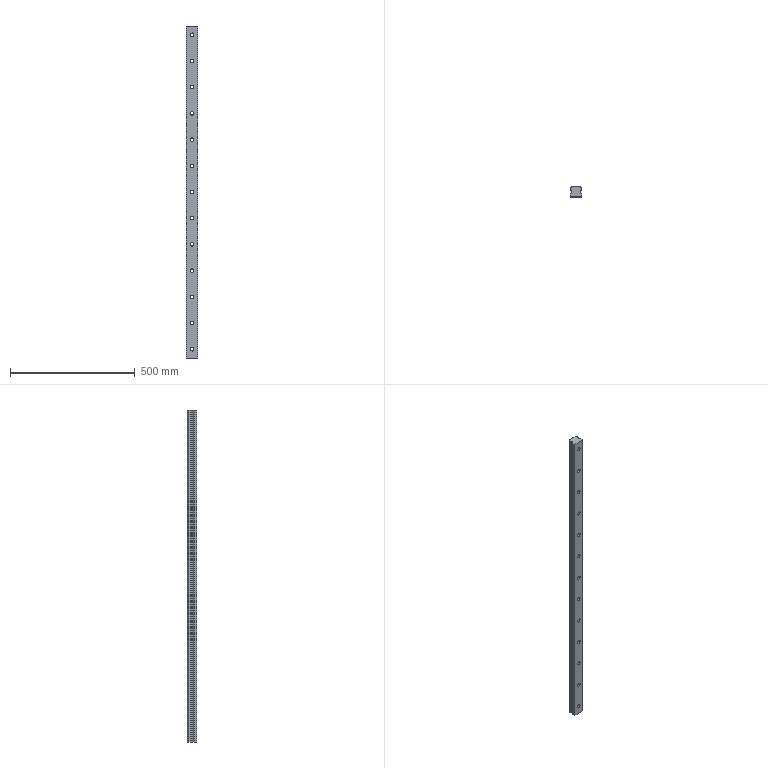Part | SolidWorks | features SplitBody 1 | 1 solid | 91 faces | box 45 x 38 x 1330 mm | volume 1945427 mm3 | cylinder 58 | plane 33 | commonest cylinder face diameters 14 x26 20 x26 3.923 x6